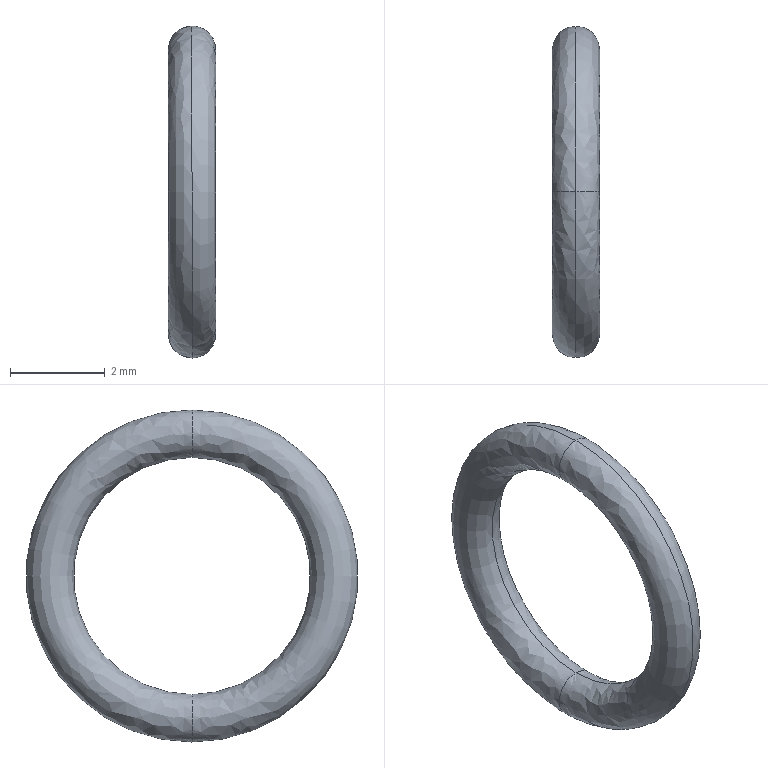Part | SolidWorks | features BaseBody 1 | 1 solid | 4 faces | box 1 x 7 x 7 mm | volume 14.803 mm3 | spline 4
STEP:
#1=CARTESIAN_POINT('',(466.537,37.715,61.866));
#2=VERTEX_POINT('',#1);
#3=CARTESIAN_POINT('',(466.537,37.715,68.866));
#4=VERTEX_POINT('',#3);
#5=CARTESIAN_POINT('',(466.537,37.715,65.366));
#6=DIRECTION('',(1.,0.,0.000000013));
#7=DIRECTION('',(-0.000000013,0.,1.));
#8=AXIS2_PLACEMENT_3D('',#5,#6,#7);
#9=CIRCLE('',#8,3.5);
#10=EDGE_CURVE('',#2,#4,#9,.T.);
#11=ORIENTED_EDGE('',*,*,#10,.F.);
#12=CARTESIAN_POINT('',(466.537,37.715,62.866));
#13=VERTEX_POINT('',#12);
#14=CARTESIAN_POINT('',(466.537,37.715,61.866));
#15=CARTESIAN_POINT('',(466.479,37.715,61.866));
#16=CARTESIAN_POINT('',(466.354,37.715,61.888));
#17=CARTESIAN_POINT('',(466.185,37.715,61.991));
#18=CARTESIAN_POINT('',(466.065,37.715,62.162));
#19=CARTESIAN_POINT('',(466.023,37.715,62.366));
#20=CARTESIAN_POINT('',(466.065,37.715,62.57));
#21=CARTESIAN_POINT('',(466.185,37.715,62.741));
#22=CARTESIAN_POINT('',(466.354,37.715,62.844));
#23=CARTESIAN_POINT('',(466.479,37.715,62.866));
#24=CARTESIAN_POINT('',(466.537,37.715,62.866));
#25=B_SPLINE_CURVE_WITH_KNOTS('',3,(#14,#15,#16,#17,#18,#19,#20,#21,#22,#23,#24),.UNSPECIFIED.,.F.,.F.,(4,1,1,1,1,1,1,1,4),(0.01923,0.125,0.25,0.375,0.5,0.625,0.75,0.875,0.9808),.UNSPECIFIED.);
#26=EDGE_CURVE('',#2,#13,#25,.T.);
#27=ORIENTED_EDGE('',*,*,#26,.T.);
#28=CARTESIAN_POINT('',(466.537,37.715,67.866));
#29=VERTEX_POINT('',#28);
#30=CARTESIAN_POINT('',(466.537,37.715,65.366));
#31=DIRECTION('',(-1.,0.,-0.000000013));
#32=DIRECTION('',(-0.000000013,0.,1.));
#33=AXIS2_PLACEMENT_3D('',#30,#31,#32);
#34=CIRCLE('',#33,2.5);
#35=EDGE_CURVE('',#29,#13,#34,.T.);
#36=ORIENTED_EDGE('',*,*,#35,.F.);
#37=CARTESIAN_POINT('',(466.537,37.715,68.866));
#38=CARTESIAN_POINT('',(466.479,37.715,68.866));
#39=CARTESIAN_POINT('',(466.354,37.715,68.844));
#40=CARTESIAN_POINT('',(466.185,37.715,68.741));
#41=CARTESIAN_POINT('',(466.065,37.715,68.57));
#42=CARTESIAN_POINT('',(466.023,37.715,68.366));
#43=CARTESIAN_POINT('',(466.065,37.715,68.162));
#44=CARTESIAN_POINT('',(466.185,37.715,67.991));
#45=CARTESIAN_POINT('',(466.354,37.715,67.888));
#46=CARTESIAN_POINT('',(466.479,37.715,67.866));
#47=CARTESIAN_POINT('',(466.537,37.715,67.866));
#48=B_SPLINE_CURVE_WITH_KNOTS('',3,(#37,#38,#39,#40,#41,#42,#43,#44,#45,#46,#47),.UNSPECIFIED.,.F.,.F.,(4,1,1,1,1,1,1,1,4),(0.01923,0.125,0.25,0.375,0.5,0.625,0.75,0.875,0.9808),.UNSPECIFIED.);
#49=EDGE_CURVE('',#4,#29,#48,.T.);
#50=ORIENTED_EDGE('',*,*,#49,.F.);
#51=EDGE_LOOP('',(#11,#27,#36,#50));
#52=FACE_OUTER_BOUND('',#51,.T.);
#53=CARTESIAN_POINT('',(466.537,37.715,68.866));
#54=CARTESIAN_POINT('',(466.537,44.715,68.866));
#55=CARTESIAN_POINT('',(466.537,44.715,61.866));
#56=CARTESIAN_POINT('',(466.537,37.715,61.866));
#57=CARTESIAN_POINT('',(466.479,37.715,68.866));
#58=CARTESIAN_POINT('',(466.479,44.715,68.866));
#59=CARTESIAN_POINT('',(466.479,44.715,61.866));
#60=CARTESIAN_POINT('',(466.479,37.715,61.866));
#61=CARTESIAN_POINT('',(466.354,37.715,68.844));
#62=CARTESIAN_POINT('',(466.354,44.671,68.844));
#63=CARTESIAN_POINT('',(466.354,44.671,61.888));
#64=CARTESIAN_POINT('',(466.354,37.715,61.888));
#65=CARTESIAN_POINT('',(466.185,37.715,68.741));
#66=CARTESIAN_POINT('',(466.185,44.464,68.741));
#67=CARTESIAN_POINT('',(466.185,44.464,61.991));
#68=CARTESIAN_POINT('',(466.185,37.715,61.991));
#69=CARTESIAN_POINT('',(466.065,37.715,68.57));
#70=CARTESIAN_POINT('',(466.065,44.123,68.57));
#71=CARTESIAN_POINT('',(466.065,44.123,62.162));
#72=CARTESIAN_POINT('',(466.065,37.715,62.162));
#73=CARTESIAN_POINT('',(466.023,37.715,68.366));
#74=CARTESIAN_POINT('',(466.023,43.715,68.366));
#75=CARTESIAN_POINT('',(466.023,43.715,62.366));
#76=CARTESIAN_POINT('',(466.023,37.715,62.366));
#77=CARTESIAN_POINT('',(466.065,37.715,68.162));
#78=CARTESIAN_POINT('',(466.065,43.306,68.162));
#79=CARTESIAN_POINT('',(466.065,43.306,62.57));
#80=CARTESIAN_POINT('',(466.065,37.715,62.57));
#81=CARTESIAN_POINT('',(466.185,37.715,67.991));
#82=CARTESIAN_POINT('',(466.185,42.965,67.991));
#83=CARTESIAN_POINT('',(466.185,42.965,62.741));
#84=CARTESIAN_POINT('',(466.185,37.715,62.741));
#85=CARTESIAN_POINT('',(466.354,37.715,67.888));
#86=CARTESIAN_POINT('',(466.354,42.758,67.888));
#87=CARTESIAN_POINT('',(466.354,42.758,62.844));
#88=CARTESIAN_POINT('',(466.354,37.715,62.844));
#89=CARTESIAN_POINT('',(466.479,37.715,67.866));
#90=CARTESIAN_POINT('',(466.479,42.715,67.866));
#91=CARTESIAN_POINT('',(466.479,42.715,62.866));
#92=CARTESIAN_POINT('',(466.479,37.715,62.866));
#93=CARTESIAN_POINT('',(466.537,37.715,67.866));
#94=CARTESIAN_POINT('',(466.537,42.715,67.866));
#95=CARTESIAN_POINT('',(466.537,42.715,62.866));
#96=CARTESIAN_POINT('',(466.537,37.715,62.866));
#97=(BOUNDED_SURFACE()B_SPLINE_SURFACE(3,3,((#53,#54,#55,#56),(#57,#58,#59,#60),(#61,#62,#63,#64),(#65,#66,#67,#68),(#69,#70,#71,#72),(#73,#74,#75,#76),(#77,#78,#79,#80),(#81,#82,#83,#84),(#85,#86,#87,#88),(#89,#90,#91,#92),(#93,#94,#95,#96)),.UNSPECIFIED.,.F.,.F.,.F.)B_SPLINE_SURFACE_WITH_KNOTS((4,1,1,1,1,1,1,1,4),(4,4),(0.01923,0.125,0.25,0.375,0.5,0.625,0.75,0.875,0.9808),(0.,1.),.UNSPECIFIED.)GEOMETRIC_REPRESENTATION_ITEM()RATIONAL_B_SPLINE_SURFACE(((1.,0.3333,0.3333,1.),(1.,0.3333,0.3333,1.),(1.,0.3333,0.3333,1.),(1.,0.3333,0.3333,1.),(1.,0.3333,0.3333,1.),(1.,0.3333,0.3333,1.),(1.,0.3333,0.3333,1.),(1.,0.3333,0.3333,1.),(1.,0.3333,0.3333,1.),(1.,0.3333,0.3333,1.),(1.,0.3333,0.3333,1.)))REPRESENTATION_ITEM('')SURFACE());
#98=ADVANCED_FACE('',(#52),#97,.F.);
#99=ORIENTED_EDGE('',*,*,#35,.T.);
#100=CARTESIAN_POINT('',(466.537,37.715,62.866));
#101=CARTESIAN_POINT('',(466.594,37.715,62.866));
#102=CARTESIAN_POINT('',(466.72,37.715,62.844));
#103=CARTESIAN_POINT('',(466.889,37.715,62.741));
#104=CARTESIAN_POINT('',(467.009,37.715,62.57));
#105=CARTESIAN_POINT('',(467.051,37.715,62.366));
#106=CARTESIAN_POINT('',(467.009,37.715,62.162));
#107=CARTESIAN_POINT('',(466.889,37.715,61.991));
#108=CARTESIAN_POINT('',(466.72,37.715,61.888));
#109=CARTESIAN_POINT('',(466.594,37.715,61.866));
#110=CARTESIAN_POINT('',(466.537,37.715,61.866));
#111=B_SPLINE_CURVE_WITH_KNOTS('',3,(#100,#101,#102,#103,#104,#105,#106,#107,#108,#109,#110),.UNSPECIFIED.,.F.,.F.,(4,1,1,1,1,1,1,1,4),(0.01923,0.125,0.25,0.375,0.5,0.625,0.75,0.875,0.9808),.UNSPECIFIED.);
#112=EDGE_CURVE('',#13,#2,#111,.T.);
#113=ORIENTED_EDGE('',*,*,#112,.T.);
#114=ORIENTED_EDGE('',*,*,#10,.T.);
#115=CARTESIAN_POINT('',(466.537,37.715,67.866));
#116=CARTESIAN_POINT('',(466.594,37.715,67.866));
#117=CARTESIAN_POINT('',(466.72,37.715,67.888));
#118=CARTESIAN_POINT('',(466.889,37.715,67.991));
#119=CARTESIAN_POINT('',(467.009,37.715,68.162));
#120=CARTESIAN_POINT('',(467.051,37.715,68.366));
#121=CARTESIAN_POINT('',(467.009,37.715,68.57));
#122=CARTESIAN_POINT('',(466.889,37.715,68.741));
#123=CARTESIAN_POINT('',(466.72,37.715,68.844));
#124=CARTESIAN_POINT('',(466.594,37.715,68.866));
#125=CARTESIAN_POINT('',(466.537,37.715,68.866));
#126=B_SPLINE_CURVE_WITH_KNOTS('',3,(#115,#116,#117,#118,#119,#120,#121,#122,#123,#124,#125),.UNSPECIFIED.,.F.,.F.,(4,1,1,1,1,1,1,1,4),(0.01923,0.125,0.25,0.375,0.5,0.625,0.75,0.875,0.9808),.UNSPECIFIED.);
#127=EDGE_CURVE('',#29,#4,#126,.T.);
#128=ORIENTED_EDGE('',*,*,#127,.F.);
#129=EDGE_LOOP('',(#99,#113,#114,#128));
#130=FACE_OUTER_BOUND('',#129,.T.);
#131=CARTESIAN_POINT('',(466.537,37.715,67.866));
#132=CARTESIAN_POINT('',(466.537,42.715,67.866));
#133=CARTESIAN_POINT('',(466.537,42.715,62.866));
#134=CARTESIAN_POINT('',(466.537,37.715,62.866));
#135=CARTESIAN_POINT('',(466.594,37.715,67.866));
#136=CARTESIAN_POINT('',(466.594,42.715,67.866));
#137=CARTESIAN_POINT('',(466.594,42.715,62.866));
#138=CARTESIAN_POINT('',(466.594,37.715,62.866));
#139=CARTESIAN_POINT('',(466.72,37.715,67.888));
#140=CARTESIAN_POINT('',(466.72,42.758,67.888));
#141=CARTESIAN_POINT('',(466.72,42.758,62.844));
#142=CARTESIAN_POINT('',(466.72,37.715,62.844));
#143=CARTESIAN_POINT('',(466.889,37.715,67.991));
#144=CARTESIAN_POINT('',(466.889,42.965,67.991));
#145=CARTESIAN_POINT('',(466.889,42.965,62.741));
#146=CARTESIAN_POINT('',(466.889,37.715,62.741));
#147=CARTESIAN_POINT('',(467.009,37.715,68.162));
#148=CARTESIAN_POINT('',(467.009,43.306,68.162));
#149=CARTESIAN_POINT('',(467.009,43.306,62.57));
#150=CARTESIAN_POINT('',(467.009,37.715,62.57));
#151=CARTESIAN_POINT('',(467.051,37.715,68.366));
#152=CARTESIAN_POINT('',(467.051,43.715,68.366));
#153=CARTESIAN_POINT('',(467.051,43.715,62.366));
#154=CARTESIAN_POINT('',(467.051,37.715,62.366));
#155=CARTESIAN_POINT('',(467.009,37.715,68.57));
#156=CARTESIAN_POINT('',(467.009,44.123,68.57));
#157=CARTESIAN_POINT('',(467.009,44.123,62.162));
#158=CARTESIAN_POINT('',(467.009,37.715,62.162));
#159=CARTESIAN_POINT('',(466.889,37.715,68.741));
#160=CARTESIAN_POINT('',(466.889,44.464,68.741));
#161=CARTESIAN_POINT('',(466.889,44.464,61.991));
#162=CARTESIAN_POINT('',(466.889,37.715,61.991));
#163=CARTESIAN_POINT('',(466.72,37.715,68.844));
#164=CARTESIAN_POINT('',(466.72,44.671,68.844));
#165=CARTESIAN_POINT('',(466.72,44.671,61.888));
#166=CARTESIAN_POINT('',(466.72,37.715,61.888));
#167=CARTESIAN_POINT('',(466.594,37.715,68.866));
#168=CARTESIAN_POINT('',(466.594,44.715,68.866));
#169=CARTESIAN_POINT('',(466.594,44.715,61.866));
#170=CARTESIAN_POINT('',(466.594,37.715,61.866));
#171=CARTESIAN_POINT('',(466.537,37.715,68.866));
#172=CARTESIAN_POINT('',(466.537,44.715,68.866));
#173=CARTESIAN_POINT('',(466.537,44.715,61.866));
#174=CARTESIAN_POINT('',(466.537,37.715,61.866));
#175=(BOUNDED_SURFACE()B_SPLINE_SURFACE(3,3,((#131,#132,#133,#134),(#135,#136,#137,#138),(#139,#140,#141,#142),(#143,#144,#145,#146),(#147,#148,#149,#150),(#151,#152,#153,#154),(#155,#156,#157,#158),(#159,#160,#161,#162),(#163,#164,#165,#166),(#167,#168,#169,#170),(#171,#172,#173,#174)),.UNSPECIFIED.,.F.,.F.,.F.)B_SPLINE_SURFACE_WITH_KNOTS((4,1,1,1,1,1,1,1,4),(4,4),(0.01923,0.125,0.25,0.375,0.5,0.625,0.75,0.875,0.9808),(0.,1.),.UNSPECIFIED.)GEOMETRIC_REPRESENTATION_ITEM()RATIONAL_B_SPLINE_SURFACE(((1.,0.3333,0.3333,1.),(1.,0.3333,0.3333,1.),(1.,0.3333,0.3333,1.),(1.,0.3333,0.3333,1.),(1.,0.3333,0.3333,1.),(1.,0.3333,0.3333,1.),(1.,0.3333,0.3333,1.),(1.,0.3333,0.3333,1.),(1.,0.3333,0.3333,1.),(1.,0.3333,0.3333,1.),(1.,0.3333,0.3333,1.)))REPRESENTATION_ITEM('')SURFACE());
#176=ADVANCED_FACE('',(#130),#175,.F.);
#177=ORIENTED_EDGE('',*,*,#26,.F.);
#178=CARTESIAN_POINT('',(466.537,37.715,65.366));
#179=DIRECTION('',(1.,0.,0.000000013));
#180=DIRECTION('',(-0.000000013,0.,1.));
#181=AXIS2_PLACEMENT_3D('',#178,#179,#180);
#182=CIRCLE('',#181,3.5);
#183=EDGE_CURVE('',#4,#2,#182,.T.);
#184=ORIENTED_EDGE('',*,*,#183,.F.);
#185=ORIENTED_EDGE('',*,*,#49,.T.);
#186=CARTESIAN_POINT('',(466.537,37.715,65.366));
#187=DIRECTION('',(-1.,0.,-0.000000013));
#188=DIRECTION('',(-0.000000013,0.,1.));
#189=AXIS2_PLACEMENT_3D('',#186,#187,#188);
#190=CIRCLE('',#189,2.5);
#191=EDGE_CURVE('',#13,#29,#190,.T.);
#192=ORIENTED_EDGE('',*,*,#191,.F.);
#193=EDGE_LOOP('',(#177,#184,#185,#192));
#194=FACE_OUTER_BOUND('',#193,.T.);
#195=CARTESIAN_POINT('',(466.537,37.715,61.866));
#196=CARTESIAN_POINT('',(466.537,30.715,61.866));
#197=CARTESIAN_POINT('',(466.537,30.715,68.866));
#198=CARTESIAN_POINT('',(466.537,37.715,68.866));
#199=CARTESIAN_POINT('',(466.479,37.715,61.866));
#200=CARTESIAN_POINT('',(466.479,30.715,61.866));
#201=CARTESIAN_POINT('',(466.479,30.715,68.866));
#202=CARTESIAN_POINT('',(466.479,37.715,68.866));
#203=CARTESIAN_POINT('',(466.354,37.715,61.888));
#204=CARTESIAN_POINT('',(466.354,30.758,61.888));
#205=CARTESIAN_POINT('',(466.354,30.758,68.844));
#206=CARTESIAN_POINT('',(466.354,37.715,68.844));
#207=CARTESIAN_POINT('',(466.185,37.715,61.991));
#208=CARTESIAN_POINT('',(466.185,30.965,61.991));
#209=CARTESIAN_POINT('',(466.185,30.965,68.741));
#210=CARTESIAN_POINT('',(466.185,37.715,68.741));
#211=CARTESIAN_POINT('',(466.065,37.715,62.162));
#212=CARTESIAN_POINT('',(466.065,31.306,62.162));
#213=CARTESIAN_POINT('',(466.065,31.306,68.57));
#214=CARTESIAN_POINT('',(466.065,37.715,68.57));
#215=CARTESIAN_POINT('',(466.023,37.715,62.366));
#216=CARTESIAN_POINT('',(466.023,31.715,62.366));
#217=CARTESIAN_POINT('',(466.023,31.715,68.366));
#218=CARTESIAN_POINT('',(466.023,37.715,68.366));
#219=CARTESIAN_POINT('',(466.065,37.715,62.57));
#220=CARTESIAN_POINT('',(466.065,32.123,62.57));
#221=CARTESIAN_POINT('',(466.065,32.123,68.162));
#222=CARTESIAN_POINT('',(466.065,37.715,68.162));
#223=CARTESIAN_POINT('',(466.185,37.715,62.741));
#224=CARTESIAN_POINT('',(466.185,32.464,62.741));
#225=CARTESIAN_POINT('',(466.185,32.464,67.991));
#226=CARTESIAN_POINT('',(466.185,37.715,67.991));
#227=CARTESIAN_POINT('',(466.354,37.715,62.844));
#228=CARTESIAN_POINT('',(466.354,32.671,62.844));
#229=CARTESIAN_POINT('',(466.354,32.671,67.888));
#230=CARTESIAN_POINT('',(466.354,37.715,67.888));
#231=CARTESIAN_POINT('',(466.479,37.715,62.866));
#232=CARTESIAN_POINT('',(466.479,32.715,62.866));
#233=CARTESIAN_POINT('',(466.479,32.715,67.866));
#234=CARTESIAN_POINT('',(466.479,37.715,67.866));
#235=CARTESIAN_POINT('',(466.537,37.715,62.866));
#236=CARTESIAN_POINT('',(466.537,32.715,62.866));
#237=CARTESIAN_POINT('',(466.537,32.715,67.866));
#238=CARTESIAN_POINT('',(466.537,37.715,67.866));
#239=(BOUNDED_SURFACE()B_SPLINE_SURFACE(3,3,((#195,#196,#197,#198),(#199,#200,#201,#202),(#203,#204,#205,#206),(#207,#208,#209,#210),(#211,#212,#213,#214),(#215,#216,#217,#218),(#219,#220,#221,#222),(#223,#224,#225,#226),(#227,#228,#229,#230),(#231,#232,#233,#234),(#235,#236,#237,#238)),.UNSPECIFIED.,.F.,.F.,.F.)B_SPLINE_SURFACE_WITH_KNOTS((4,1,1,1,1,1,1,1,4),(4,4),(0.01923,0.125,0.25,0.375,0.5,0.625,0.75,0.875,0.9808),(0.,1.),.UNSPECIFIED.)GEOMETRIC_REPRESENTATION_ITEM()RATIONAL_B_SPLINE_SURFACE(((1.,0.3333,0.3333,1.),(1.,0.3333,0.3333,1.),(1.,0.3333,0.3333,1.),(1.,0.3333,0.3333,1.),(1.,0.3333,0.3333,1.),(1.,0.3333,0.3333,1.),(1.,0.3333,0.3333,1.),(1.,0.3333,0.3333,1.),(1.,0.3333,0.3333,1.),(1.,0.3333,0.3333,1.),(1.,0.3333,0.3333,1.)))REPRESENTATION_ITEM('')SURFACE());
#240=ADVANCED_FACE('',(#194),#239,.F.);
#241=ORIENTED_EDGE('',*,*,#112,.F.);
#242=ORIENTED_EDGE('',*,*,#191,.T.);
#243=ORIENTED_EDGE('',*,*,#127,.T.);
#244=ORIENTED_EDGE('',*,*,#183,.T.);
#245=EDGE_LOOP('',(#241,#242,#243,#244));
#246=FACE_OUTER_BOUND('',#245,.T.);
#247=CARTESIAN_POINT('',(466.537,37.715,62.866));
#248=CARTESIAN_POINT('',(466.537,32.715,62.866));
#249=CARTESIAN_POINT('',(466.537,32.715,67.866));
#250=CARTESIAN_POINT('',(466.537,37.715,67.866));
#251=CARTESIAN_POINT('',(466.594,37.715,62.866));
#252=CARTESIAN_POINT('',(466.594,32.715,62.866));
#253=CARTESIAN_POINT('',(466.594,32.715,67.866));
#254=CARTESIAN_POINT('',(466.594,37.715,67.866));
#255=CARTESIAN_POINT('',(466.72,37.715,62.844));
#256=CARTESIAN_POINT('',(466.72,32.671,62.844));
#257=CARTESIAN_POINT('',(466.72,32.671,67.888));
#258=CARTESIAN_POINT('',(466.72,37.715,67.888));
#259=CARTESIAN_POINT('',(466.889,37.715,62.741));
#260=CARTESIAN_POINT('',(466.889,32.464,62.741));
#261=CARTESIAN_POINT('',(466.889,32.464,67.991));
#262=CARTESIAN_POINT('',(466.889,37.715,67.991));
#263=CARTESIAN_POINT('',(467.009,37.715,62.57));
#264=CARTESIAN_POINT('',(467.009,32.123,62.57));
#265=CARTESIAN_POINT('',(467.009,32.123,68.162));
#266=CARTESIAN_POINT('',(467.009,37.715,68.162));
#267=CARTESIAN_POINT('',(467.051,37.715,62.366));
#268=CARTESIAN_POINT('',(467.051,31.715,62.366));
#269=CARTESIAN_POINT('',(467.051,31.715,68.366));
#270=CARTESIAN_POINT('',(467.051,37.715,68.366));
#271=CARTESIAN_POINT('',(467.009,37.715,62.162));
#272=CARTESIAN_POINT('',(467.009,31.306,62.162));
#273=CARTESIAN_POINT('',(467.009,31.306,68.57));
#274=CARTESIAN_POINT('',(467.009,37.715,68.57));
#275=CARTESIAN_POINT('',(466.889,37.715,61.991));
#276=CARTESIAN_POINT('',(466.889,30.965,61.991));
#277=CARTESIAN_POINT('',(466.889,30.965,68.741));
#278=CARTESIAN_POINT('',(466.889,37.715,68.741));
#279=CARTESIAN_POINT('',(466.72,37.715,61.888));
#280=CARTESIAN_POINT('',(466.72,30.758,61.888));
#281=CARTESIAN_POINT('',(466.72,30.758,68.844));
#282=CARTESIAN_POINT('',(466.72,37.715,68.844));
#283=CARTESIAN_POINT('',(466.594,37.715,61.866));
#284=CARTESIAN_POINT('',(466.594,30.715,61.866));
#285=CARTESIAN_POINT('',(466.594,30.715,68.866));
#286=CARTESIAN_POINT('',(466.594,37.715,68.866));
#287=CARTESIAN_POINT('',(466.537,37.715,61.866));
#288=CARTESIAN_POINT('',(466.537,30.715,61.866));
#289=CARTESIAN_POINT('',(466.537,30.715,68.866));
#290=CARTESIAN_POINT('',(466.537,37.715,68.866));
#291=(BOUNDED_SURFACE()B_SPLINE_SURFACE(3,3,((#247,#248,#249,#250),(#251,#252,#253,#254),(#255,#256,#257,#258),(#259,#260,#261,#262),(#263,#264,#265,#266),(#267,#268,#269,#270),(#271,#272,#273,#274),(#275,#276,#277,#278),(#279,#280,#281,#282),(#283,#284,#285,#286),(#287,#288,#289,#290)),.UNSPECIFIED.,.F.,.F.,.F.)B_SPLINE_SURFACE_WITH_KNOTS((4,1,1,1,1,1,1,1,4),(4,4),(0.01923,0.125,0.25,0.375,0.5,0.625,0.75,0.875,0.9808),(0.,1.),.UNSPECIFIED.)GEOMETRIC_REPRESENTATION_ITEM()RATIONAL_B_SPLINE_SURFACE(((1.,0.3333,0.3333,1.),(1.,0.3333,0.3333,1.),(1.,0.3333,0.3333,1.),(1.,0.3333,0.3333,1.),(1.,0.3333,0.3333,1.),(1.,0.3333,0.3333,1.),(1.,0.3333,0.3333,1.),(1.,0.3333,0.3333,1.),(1.,0.3333,0.3333,1.),(1.,0.3333,0.3333,1.),(1.,0.3333,0.3333,1.)))REPRESENTATION_ITEM('')SURFACE());
#292=ADVANCED_FACE('',(#246),#291,.F.);
#293=CLOSED_SHELL('',(#98,#176,#240,#292));
#294=MANIFOLD_SOLID_BREP('',#293);
#295=CARTESIAN_POINT('',(0.,0.,0.));
#296=DIRECTION('',(0.,0.,1.));
#297=DIRECTION('',(1.,0.,0.));
#298=AXIS2_PLACEMENT_3D('',#295,#296,#297);
#299=(LENGTH_UNIT()NAMED_UNIT(*)SI_UNIT(.MILLI.,.METRE.));
#300=UNCERTAINTY_MEASURE_WITH_UNIT(LENGTH_MEASURE(0.00001),#299,'','');
#301=(NAMED_UNIT(*)PLANE_ANGLE_UNIT()SI_UNIT($,.RADIAN.));
#302=(NAMED_UNIT(*)SI_UNIT($,.STERADIAN.)SOLID_ANGLE_UNIT());
#303=(GEOMETRIC_REPRESENTATION_CONTEXT(3)GLOBAL_UNCERTAINTY_ASSIGNED_CONTEXT((#300))GLOBAL_UNIT_ASSIGNED_CONTEXT((#299,#301,#302))REPRESENTATION_CONTEXT('',''));
#304=ADVANCED_BREP_SHAPE_REPRESENTATION('',(#294,#298),#303);